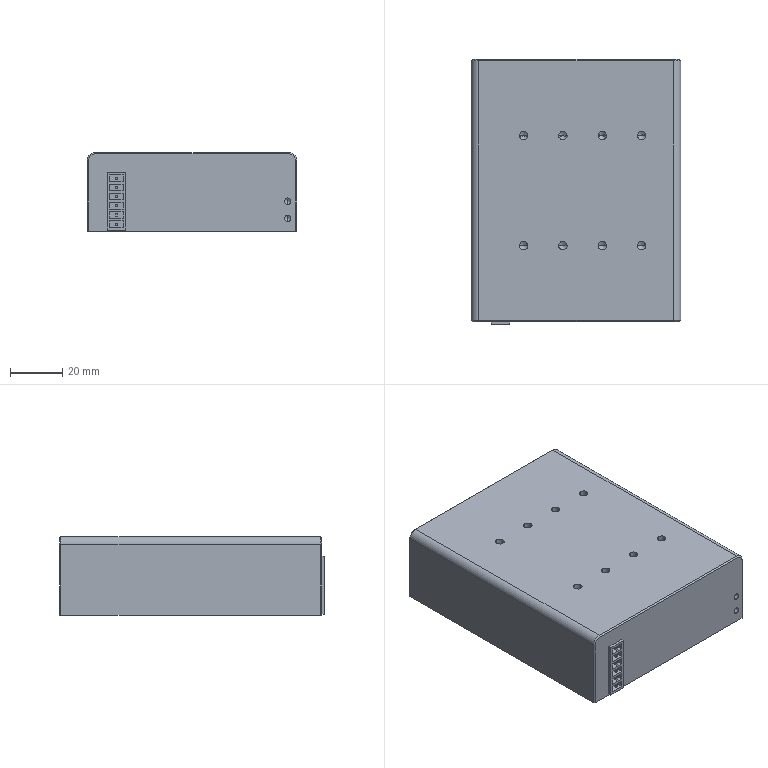Part | NX | features BREP 7 | 7 solids | 147 faces | box 80 x 101 x 30 mm | volume 238985 mm3 | plane 89 | cylinder 34 | cone 24 | commonest cylinder face diameters 3.242 x16 0.5 x12 2.459 x4 6 x2